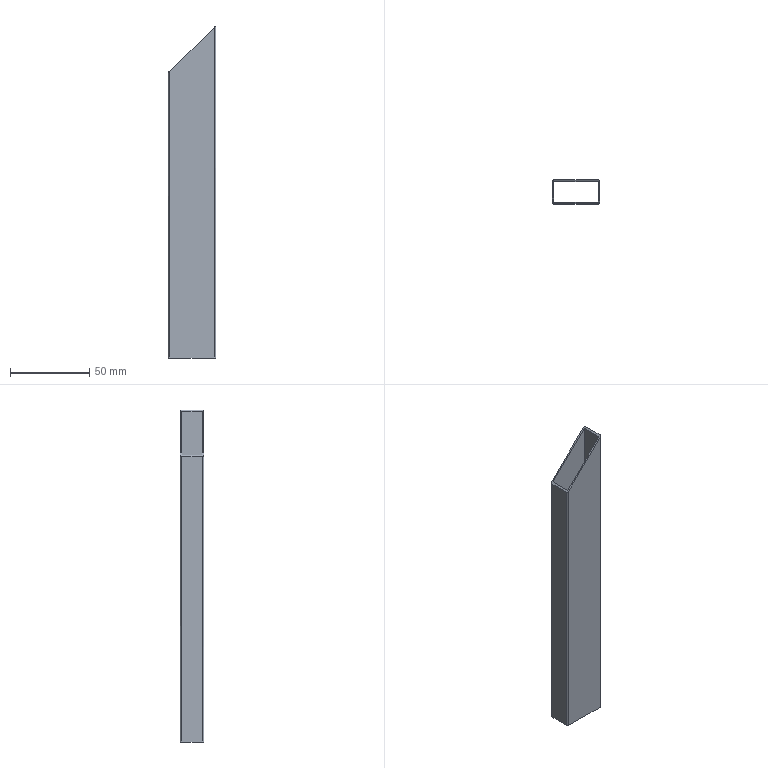Part | STEP file | Q7C1208 | 1 solid | 14 faces | box 30 x 15 x 209.35 mm | volume 16574 mm3 | plane 10 | cylinder 4 | commonest cylinder face diameters 2 x4
STEP:
#1=CARTESIAN_POINT('',(0.,0.,0.));
#2=DIRECTION('',(0.,0.,1.));
#3=DIRECTION('',(1.,0.,0.));
#4=AXIS2_PLACEMENT_3D('',#1,#2,#3);
#5=CARTESIAN_POINT('',(15.,6.5,209.35));
#6=VERTEX_POINT('',#5);
#7=CARTESIAN_POINT('',(14.,7.5,208.371));
#8=VERTEX_POINT('',#7);
#9=CARTESIAN_POINT('',(15.,6.5,209.35));
#10=CARTESIAN_POINT('',(15.,7.086,209.35));
#11=CARTESIAN_POINT('',(14.586,7.5,208.944));
#12=CARTESIAN_POINT('',(14.,7.5,208.371));
#13=(BOUNDED_CURVE()B_SPLINE_CURVE(3,(#9,#10,#11,#12),.UNSPECIFIED.,.F.,.F.)B_SPLINE_CURVE_WITH_KNOTS((4,4),(3.142,4.712),.PIECEWISE_BEZIER_KNOTS.)CURVE()GEOMETRIC_REPRESENTATION_ITEM()RATIONAL_B_SPLINE_CURVE((1.,0.8047,0.8047,1.))REPRESENTATION_ITEM(''));
#14=CARTESIAN_POINT('',(14.,6.5,230.));
#15=DIRECTION('',(0.,0.,-1.));
#16=DIRECTION('',(-1.,0.,0.));
#17=AXIS2_PLACEMENT_3D('',#14,#15,#16);
#18=CYLINDRICAL_SURFACE('',#17,1.);
#19=CARTESIAN_POINT('',(3.142,20.65));
#20=CARTESIAN_POINT('',(3.12,20.65));
#21=CARTESIAN_POINT('',(3.077,20.652));
#22=CARTESIAN_POINT('',(3.01,20.658));
#23=CARTESIAN_POINT('',(2.942,20.669));
#24=CARTESIAN_POINT('',(2.872,20.685));
#25=CARTESIAN_POINT('',(2.801,20.706));
#26=CARTESIAN_POINT('',(2.729,20.732));
#27=CARTESIAN_POINT('',(2.655,20.763));
#28=CARTESIAN_POINT('',(2.581,20.799));
#29=CARTESIAN_POINT('',(2.507,20.84));
#30=CARTESIAN_POINT('',(2.432,20.886));
#31=CARTESIAN_POINT('',(2.356,20.936));
#32=CARTESIAN_POINT('',(2.281,20.991));
#33=CARTESIAN_POINT('',(2.206,21.048));
#34=CARTESIAN_POINT('',(2.131,21.109));
#35=CARTESIAN_POINT('',(2.057,21.171));
#36=CARTESIAN_POINT('',(1.984,21.236));
#37=CARTESIAN_POINT('',(1.912,21.302));
#38=CARTESIAN_POINT('',(1.841,21.368));
#39=CARTESIAN_POINT('',(1.771,21.435));
#40=CARTESIAN_POINT('',(1.702,21.501));
#41=CARTESIAN_POINT('',(1.636,21.566));
#42=CARTESIAN_POINT('',(1.592,21.608));
#43=CARTESIAN_POINT('',(1.571,21.629));
#44=B_SPLINE_CURVE_WITH_KNOTS('',3,(#19,#20,#21,#22,#23,#24,#25,#26,#27,#28,#29,#30,#31,#32,#33,#34,#35,#36,#37,#38,#39,#40,#41,#42,#43),.UNSPECIFIED.,.F.,.F.,(4,1,1,1,1,1,1,1,1,1,1,1,1,1,1,1,1,1,1,1,1,1,4),(3.142,3.213,3.284,3.356,3.427,3.499,3.57,3.641,3.713,3.784,3.856,3.927,3.998,4.07,4.141,4.213,4.284,4.355,4.427,4.498,4.57,4.641,4.712),.QUASI_UNIFORM_KNOTS.);
#45=(GEOMETRIC_REPRESENTATION_CONTEXT(2)PARAMETRIC_REPRESENTATION_CONTEXT()REPRESENTATION_CONTEXT('',''));
#46=DEFINITIONAL_REPRESENTATION('',(#44),#45);
#47=PCURVE('',#18,#46);
#48=CARTESIAN_POINT('',(16.518,298.041,210.835));
#49=DIRECTION('',(-0.6995,0.,0.7146));
#50=DIRECTION('',(0.7146,0.,0.6995));
#51=AXIS2_PLACEMENT_3D('',#48,#49,#50);
#52=PLANE('',#51);
#53=CARTESIAN_POINT('',(-2.124,-291.541));
#54=CARTESIAN_POINT('',(-2.124,-290.955));
#55=CARTESIAN_POINT('',(-2.703,-290.541));
#56=CARTESIAN_POINT('',(-3.523,-290.541));
#57=(BOUNDED_CURVE()B_SPLINE_CURVE(3,(#53,#54,#55,#56),.UNSPECIFIED.,.F.,.F.)B_SPLINE_CURVE_WITH_KNOTS((4,4),(3.142,4.712),.PIECEWISE_BEZIER_KNOTS.)CURVE()GEOMETRIC_REPRESENTATION_ITEM()RATIONAL_B_SPLINE_CURVE((1.,0.8047,0.8047,1.))REPRESENTATION_ITEM(''));
#58=(GEOMETRIC_REPRESENTATION_CONTEXT(2)PARAMETRIC_REPRESENTATION_CONTEXT()REPRESENTATION_CONTEXT('',''));
#59=DEFINITIONAL_REPRESENTATION('',(#57),#58);
#60=PCURVE('',#52,#59);
#61=SURFACE_CURVE('',#13,(#47,#60),.PCURVE_S1.);
#62=EDGE_CURVE('',#6,#8,#61,.T.);
#63=ORIENTED_EDGE('',*,*,#62,.F.);
#64=CARTESIAN_POINT('',(15.,6.5,0.));
#65=VERTEX_POINT('',#64);
#66=CARTESIAN_POINT('',(15.,6.5,230.));
#67=DIRECTION('',(0.,0.,-1.));
#68=VECTOR('',#67,1.);
#69=LINE('',#66,#68);
#70=CARTESIAN_POINT('',(3.142,0.));
#71=DIRECTION('',(0.,1.));
#72=VECTOR('',#71,1.);
#73=LINE('',#70,#72);
#74=(GEOMETRIC_REPRESENTATION_CONTEXT(2)PARAMETRIC_REPRESENTATION_CONTEXT()REPRESENTATION_CONTEXT('',''));
#75=DEFINITIONAL_REPRESENTATION('',(#73),#74);
#76=PCURVE('',#18,#75);
#77=CARTESIAN_POINT('',(15.,6.5,230.));
#78=DIRECTION('',(-1.,0.,0.));
#79=DIRECTION('',(0.,0.,1.));
#80=AXIS2_PLACEMENT_3D('',#77,#78,#79);
#81=PLANE('',#80);
#82=CARTESIAN_POINT('',(0.,0.));
#83=DIRECTION('',(-1.,0.));
#84=VECTOR('',#83,1.);
#85=LINE('',#82,#84);
#86=(GEOMETRIC_REPRESENTATION_CONTEXT(2)PARAMETRIC_REPRESENTATION_CONTEXT()REPRESENTATION_CONTEXT('',''));
#87=DEFINITIONAL_REPRESENTATION('',(#85),#86);
#88=PCURVE('',#81,#87);
#89=SURFACE_CURVE('',#69,(#76,#88),.PCURVE_S1.);
#90=EDGE_CURVE('',#6,#65,#89,.T.);
#91=ORIENTED_EDGE('',*,*,#90,.T.);
#92=CARTESIAN_POINT('',(14.,7.5,0.));
#93=VERTEX_POINT('',#92);
#94=CARTESIAN_POINT('',(14.,6.5,0.));
#95=DIRECTION('',(0.,0.,1.));
#96=DIRECTION('',(-1.,0.,0.));
#97=AXIS2_PLACEMENT_3D('',#94,#95,#96);
#98=CIRCLE('',#97,1.);
#99=CARTESIAN_POINT('',(6.283,230.));
#100=DIRECTION('',(-1.,0.));
#101=VECTOR('',#100,1.);
#102=LINE('',#99,#101);
#103=(GEOMETRIC_REPRESENTATION_CONTEXT(2)PARAMETRIC_REPRESENTATION_CONTEXT()REPRESENTATION_CONTEXT('',''));
#104=DEFINITIONAL_REPRESENTATION('',(#102),#103);
#105=PCURVE('',#18,#104);
#106=CARTESIAN_POINT('',(14.,6.5,0.));
#107=DIRECTION('',(0.,0.,-1.));
#108=DIRECTION('',(-1.,0.,0.));
#109=AXIS2_PLACEMENT_3D('',#106,#107,#108);
#110=PLANE('',#109);
#111=CARTESIAN_POINT('',(1.,0.));
#112=CARTESIAN_POINT('',(1.,-1.732));
#113=CARTESIAN_POINT('',(-0.5,-0.866));
#114=CARTESIAN_POINT('',(-2.,0.));
#115=CARTESIAN_POINT('',(-0.5,0.866));
#116=CARTESIAN_POINT('',(1.,1.732));
#117=CARTESIAN_POINT('',(1.,0.));
#118=(BOUNDED_CURVE()B_SPLINE_CURVE(2,(#111,#112,#113,#114,#115,#116,#117),.UNSPECIFIED.,.T.,.F.)B_SPLINE_CURVE_WITH_KNOTS((1,2,2,2,2,1),(-2.094,0.,2.094,4.189,6.283,8.378),.UNSPECIFIED.)CURVE()GEOMETRIC_REPRESENTATION_ITEM()RATIONAL_B_SPLINE_CURVE((1.,0.5,1.,0.5,1.,0.5,1.))REPRESENTATION_ITEM(''));
#119=(GEOMETRIC_REPRESENTATION_CONTEXT(2)PARAMETRIC_REPRESENTATION_CONTEXT()REPRESENTATION_CONTEXT('',''));
#120=DEFINITIONAL_REPRESENTATION('',(#118),#119);
#121=PCURVE('',#110,#120);
#122=SURFACE_CURVE('',#98,(#105,#121),.PCURVE_S1.);
#123=EDGE_CURVE('',#65,#93,#122,.T.);
#124=ORIENTED_EDGE('',*,*,#123,.T.);
#125=CARTESIAN_POINT('',(14.,7.5,230.));
#126=DIRECTION('',(0.,0.,-1.));
#127=VECTOR('',#126,1.);
#128=LINE('',#125,#127);
#129=CARTESIAN_POINT('',(1.571,0.));
#130=DIRECTION('',(0.,1.));
#131=VECTOR('',#130,1.);
#132=LINE('',#129,#131);
#133=(GEOMETRIC_REPRESENTATION_CONTEXT(2)PARAMETRIC_REPRESENTATION_CONTEXT()REPRESENTATION_CONTEXT('',''));
#134=DEFINITIONAL_REPRESENTATION('',(#132),#133);
#135=PCURVE('',#18,#134);
#136=CARTESIAN_POINT('',(-14.,7.5,230.));
#137=DIRECTION('',(0.,-1.,0.));
#138=DIRECTION('',(0.,0.,-1.));
#139=AXIS2_PLACEMENT_3D('',#136,#137,#138);
#140=PLANE('',#139);
#141=CARTESIAN_POINT('',(0.,28.));
#142=DIRECTION('',(1.,0.));
#143=VECTOR('',#142,1.);
#144=LINE('',#141,#143);
#145=(GEOMETRIC_REPRESENTATION_CONTEXT(2)PARAMETRIC_REPRESENTATION_CONTEXT()REPRESENTATION_CONTEXT('',''));
#146=DEFINITIONAL_REPRESENTATION('',(#144),#145);
#147=PCURVE('',#140,#146);
#148=SURFACE_CURVE('',#128,(#135,#147),.PCURVE_S1.);
#149=EDGE_CURVE('',#8,#93,#148,.T.);
#150=ORIENTED_EDGE('',*,*,#149,.F.);
#151=EDGE_LOOP('',(#63,#91,#124,#150));
#152=FACE_BOUND('',#151,.T.);
#153=ADVANCED_FACE('',(#152),#18,.T.);
#154=CARTESIAN_POINT('',(-14.,7.5,180.963));
#155=VERTEX_POINT('',#154);
#156=CARTESIAN_POINT('',(10.513,7.5,204.958));
#157=DIRECTION('',(-0.7146,0.,-0.6995));
#158=VECTOR('',#157,1.);
#159=LINE('',#156,#158);
#160=CARTESIAN_POINT('',(25.042,24.513));
#161=DIRECTION('',(0.6995,-0.7146));
#162=VECTOR('',#161,1.);
#163=LINE('',#160,#162);
#164=(GEOMETRIC_REPRESENTATION_CONTEXT(2)PARAMETRIC_REPRESENTATION_CONTEXT()REPRESENTATION_CONTEXT('',''));
#165=DEFINITIONAL_REPRESENTATION('',(#163),#164);
#166=PCURVE('',#140,#165);
#167=CARTESIAN_POINT('',(-8.403,-290.541));
#168=DIRECTION('',(-1.,0.));
#169=VECTOR('',#168,1.);
#170=LINE('',#167,#169);
#171=(GEOMETRIC_REPRESENTATION_CONTEXT(2)PARAMETRIC_REPRESENTATION_CONTEXT()REPRESENTATION_CONTEXT('',''));
#172=DEFINITIONAL_REPRESENTATION('',(#170),#171);
#173=PCURVE('',#52,#172);
#174=SURFACE_CURVE('',#159,(#166,#173),.PCURVE_S1.);
#175=EDGE_CURVE('',#8,#155,#174,.T.);
#176=ORIENTED_EDGE('',*,*,#175,.F.);
#177=ORIENTED_EDGE('',*,*,#149,.T.);
#178=CARTESIAN_POINT('',(-14.,7.5,0.));
#179=VERTEX_POINT('',#178);
#180=CARTESIAN_POINT('',(-14.,7.5,0.));
#181=DIRECTION('',(-1.,0.,0.));
#182=VECTOR('',#181,1.);
#183=LINE('',#180,#182);
#184=CARTESIAN_POINT('',(230.,0.));
#185=DIRECTION('',(0.,-1.));
#186=VECTOR('',#185,1.);
#187=LINE('',#184,#186);
#188=(GEOMETRIC_REPRESENTATION_CONTEXT(2)PARAMETRIC_REPRESENTATION_CONTEXT()REPRESENTATION_CONTEXT('',''));
#189=DEFINITIONAL_REPRESENTATION('',(#187),#188);
#190=PCURVE('',#140,#189);
#191=CARTESIAN_POINT('',(28.,1.));
#192=DIRECTION('',(1.,0.));
#193=VECTOR('',#192,1.);
#194=LINE('',#191,#193);
#195=(GEOMETRIC_REPRESENTATION_CONTEXT(2)PARAMETRIC_REPRESENTATION_CONTEXT()REPRESENTATION_CONTEXT('',''));
#196=DEFINITIONAL_REPRESENTATION('',(#194),#195);
#197=PCURVE('',#110,#196);
#198=SURFACE_CURVE('',#183,(#190,#197),.PCURVE_S1.);
#199=EDGE_CURVE('',#93,#179,#198,.T.);
#200=ORIENTED_EDGE('',*,*,#199,.T.);
#201=CARTESIAN_POINT('',(-14.,7.5,230.));
#202=DIRECTION('',(0.,0.,-1.));
#203=VECTOR('',#202,1.);
#204=LINE('',#201,#203);
#205=CARTESIAN_POINT('',(0.,0.));
#206=DIRECTION('',(1.,0.));
#207=VECTOR('',#206,1.);
#208=LINE('',#205,#207);
#209=(GEOMETRIC_REPRESENTATION_CONTEXT(2)PARAMETRIC_REPRESENTATION_CONTEXT()REPRESENTATION_CONTEXT('',''));
#210=DEFINITIONAL_REPRESENTATION('',(#208),#209);
#211=PCURVE('',#140,#210);
#212=CARTESIAN_POINT('',(-14.,6.5,230.));
#213=DIRECTION('',(0.,0.,-1.));
#214=DIRECTION('',(-1.,0.,0.));
#215=AXIS2_PLACEMENT_3D('',#212,#213,#214);
#216=CYLINDRICAL_SURFACE('',#215,1.);
#217=CARTESIAN_POINT('',(1.571,0.));
#218=DIRECTION('',(0.,1.));
#219=VECTOR('',#218,1.);
#220=LINE('',#217,#219);
#221=(GEOMETRIC_REPRESENTATION_CONTEXT(2)PARAMETRIC_REPRESENTATION_CONTEXT()REPRESENTATION_CONTEXT('',''));
#222=DEFINITIONAL_REPRESENTATION('',(#220),#221);
#223=PCURVE('',#216,#222);
#224=SURFACE_CURVE('',#204,(#211,#223),.PCURVE_S1.);
#225=EDGE_CURVE('',#155,#179,#224,.T.);
#226=ORIENTED_EDGE('',*,*,#225,.F.);
#227=EDGE_LOOP('',(#176,#177,#200,#226));
#228=FACE_BOUND('',#227,.T.);
#229=ADVANCED_FACE('',(#228),#140,.F.);
#230=CARTESIAN_POINT('',(-15.,6.5,179.984));
#231=VERTEX_POINT('',#230);
#232=CARTESIAN_POINT('',(-14.,7.5,180.963));
#233=CARTESIAN_POINT('',(-14.586,7.5,180.389));
#234=CARTESIAN_POINT('',(-15.,7.086,179.984));
#235=CARTESIAN_POINT('',(-15.,6.5,179.984));
#236=(BOUNDED_CURVE()B_SPLINE_CURVE(3,(#232,#233,#234,#235),.UNSPECIFIED.,.F.,.F.)B_SPLINE_CURVE_WITH_KNOTS((4,4),(4.712,6.283),.PIECEWISE_BEZIER_KNOTS.)CURVE()GEOMETRIC_REPRESENTATION_ITEM()RATIONAL_B_SPLINE_CURVE((1.,0.8047,0.8047,1.))REPRESENTATION_ITEM(''));
#237=CARTESIAN_POINT('',(1.571,49.037));
#238=CARTESIAN_POINT('',(1.549,49.058));
#239=CARTESIAN_POINT('',(1.506,49.101));
#240=CARTESIAN_POINT('',(1.439,49.166));
#241=CARTESIAN_POINT('',(1.371,49.232));
#242=CARTESIAN_POINT('',(1.301,49.298));
#243=CARTESIAN_POINT('',(1.23,49.365));
#244=CARTESIAN_POINT('',(1.158,49.431));
#245=CARTESIAN_POINT('',(1.085,49.495));
#246=CARTESIAN_POINT('',(1.01,49.558));
#247=CARTESIAN_POINT('',(0.9358,49.619));
#248=CARTESIAN_POINT('',(0.8607,49.676));
#249=CARTESIAN_POINT('',(0.7854,49.73));
#250=CARTESIAN_POINT('',(0.7101,49.78));
#251=CARTESIAN_POINT('',(0.635,49.826));
#252=CARTESIAN_POINT('',(0.5603,49.867));
#253=CARTESIAN_POINT('',(0.4863,49.904));
#254=CARTESIAN_POINT('',(0.413,49.935));
#255=CARTESIAN_POINT('',(0.3408,49.961));
#256=CARTESIAN_POINT('',(0.2697,49.982));
#257=CARTESIAN_POINT('',(0.2,49.997));
#258=CARTESIAN_POINT('',(0.1316,50.008));
#259=CARTESIAN_POINT('',(0.06485,50.015));
#260=CARTESIAN_POINT('',(0.02143,50.016));
#261=CARTESIAN_POINT('',(0.,50.016));
#262=B_SPLINE_CURVE_WITH_KNOTS('',3,(#237,#238,#239,#240,#241,#242,#243,#244,#245,#246,#247,#248,#249,#250,#251,#252,#253,#254,#255,#256,#257,#258,#259,#260,#261),.UNSPECIFIED.,.F.,.F.,(4,1,1,1,1,1,1,1,1,1,1,1,1,1,1,1,1,1,1,1,1,1,4),(4.712,4.784,4.855,4.927,4.998,5.069,5.141,5.212,5.284,5.355,5.426,5.498,5.569,5.641,5.712,5.783,5.855,5.926,5.998,6.069,6.14,6.212,6.283),.QUASI_UNIFORM_KNOTS.);
#263=(GEOMETRIC_REPRESENTATION_CONTEXT(2)PARAMETRIC_REPRESENTATION_CONTEXT()REPRESENTATION_CONTEXT('',''));
#264=DEFINITIONAL_REPRESENTATION('',(#262),#263);
#265=PCURVE('',#216,#264);
#266=CARTESIAN_POINT('',(-42.705,-290.541));
#267=CARTESIAN_POINT('',(-43.525,-290.541));
#268=CARTESIAN_POINT('',(-44.104,-290.955));
#269=CARTESIAN_POINT('',(-44.104,-291.541));
#270=(BOUNDED_CURVE()B_SPLINE_CURVE(3,(#266,#267,#268,#269),.UNSPECIFIED.,.F.,.F.)B_SPLINE_CURVE_WITH_KNOTS((4,4),(4.712,6.283),.PIECEWISE_BEZIER_KNOTS.)CURVE()GEOMETRIC_REPRESENTATION_ITEM()RATIONAL_B_SPLINE_CURVE((1.,0.8047,0.8047,1.))REPRESENTATION_ITEM(''));
#271=(GEOMETRIC_REPRESENTATION_CONTEXT(2)PARAMETRIC_REPRESENTATION_CONTEXT()REPRESENTATION_CONTEXT('',''));
#272=DEFINITIONAL_REPRESENTATION('',(#270),#271);
#273=PCURVE('',#52,#272);
#274=SURFACE_CURVE('',#236,(#265,#273),.PCURVE_S1.);
#275=EDGE_CURVE('',#155,#231,#274,.T.);
#276=ORIENTED_EDGE('',*,*,#275,.F.);
#277=ORIENTED_EDGE('',*,*,#225,.T.);
#278=CARTESIAN_POINT('',(-15.,6.5,0.));
#279=VERTEX_POINT('',#278);
#280=CARTESIAN_POINT('',(-14.,6.5,0.));
#281=DIRECTION('',(0.,0.,1.));
#282=DIRECTION('',(1.,0.,0.));
#283=AXIS2_PLACEMENT_3D('',#280,#281,#282);
#284=CIRCLE('',#283,1.);
#285=CARTESIAN_POINT('',(3.142,230.));
#286=DIRECTION('',(-1.,0.));
#287=VECTOR('',#286,1.);
#288=LINE('',#285,#287);
#289=(GEOMETRIC_REPRESENTATION_CONTEXT(2)PARAMETRIC_REPRESENTATION_CONTEXT()REPRESENTATION_CONTEXT('',''));
#290=DEFINITIONAL_REPRESENTATION('',(#288),#289);
#291=PCURVE('',#216,#290);
#292=CARTESIAN_POINT('',(27.,0.));
#293=CARTESIAN_POINT('',(27.,1.732));
#294=CARTESIAN_POINT('',(28.5,0.866));
#295=CARTESIAN_POINT('',(30.,0.));
#296=CARTESIAN_POINT('',(28.5,-0.866));
#297=CARTESIAN_POINT('',(27.,-1.732));
#298=CARTESIAN_POINT('',(27.,0.));
#299=(BOUNDED_CURVE()B_SPLINE_CURVE(2,(#292,#293,#294,#295,#296,#297,#298),.UNSPECIFIED.,.T.,.F.)B_SPLINE_CURVE_WITH_KNOTS((1,2,2,2,2,1),(-2.094,0.,2.094,4.189,6.283,8.378),.UNSPECIFIED.)CURVE()GEOMETRIC_REPRESENTATION_ITEM()RATIONAL_B_SPLINE_CURVE((1.,0.5,1.,0.5,1.,0.5,1.))REPRESENTATION_ITEM(''));
#300=(GEOMETRIC_REPRESENTATION_CONTEXT(2)PARAMETRIC_REPRESENTATION_CONTEXT()REPRESENTATION_CONTEXT('',''));
#301=DEFINITIONAL_REPRESENTATION('',(#299),#300);
#302=PCURVE('',#110,#301);
#303=SURFACE_CURVE('',#284,(#291,#302),.PCURVE_S1.);
#304=EDGE_CURVE('',#179,#279,#303,.T.);
#305=ORIENTED_EDGE('',*,*,#304,.T.);
#306=CARTESIAN_POINT('',(-15.,6.5,230.));
#307=DIRECTION('',(0.,0.,-1.));
#308=VECTOR('',#307,1.);
#309=LINE('',#306,#308);
#310=CARTESIAN_POINT('',(0.,0.));
#311=DIRECTION('',(0.,1.));
#312=VECTOR('',#311,1.);
#313=LINE('',#310,#312);
#314=(GEOMETRIC_REPRESENTATION_CONTEXT(2)PARAMETRIC_REPRESENTATION_CONTEXT()REPRESENTATION_CONTEXT('',''));
#315=DEFINITIONAL_REPRESENTATION('',(#313),#314);
#316=PCURVE('',#216,#315);
#317=CARTESIAN_POINT('',(-15.,6.5,230.));
#318=DIRECTION('',(1.,0.,0.));
#319=DIRECTION('',(0.,1.,0.));
#320=AXIS2_PLACEMENT_3D('',#317,#318,#319);
#321=PLANE('',#320);
#322=CARTESIAN_POINT('',(0.,0.));
#323=DIRECTION('',(0.,-1.));
#324=VECTOR('',#323,1.);
#325=LINE('',#322,#324);
#326=(GEOMETRIC_REPRESENTATION_CONTEXT(2)PARAMETRIC_REPRESENTATION_CONTEXT()REPRESENTATION_CONTEXT('',''));
#327=DEFINITIONAL_REPRESENTATION('',(#325),#326);
#328=PCURVE('',#321,#327);
#329=SURFACE_CURVE('',#309,(#316,#328),.PCURVE_S1.);
#330=EDGE_CURVE('',#231,#279,#329,.T.);
#331=ORIENTED_EDGE('',*,*,#330,.F.);
#332=EDGE_LOOP('',(#276,#277,#305,#331));
#333=FACE_BOUND('',#332,.T.);
#334=ADVANCED_FACE('',(#333),#216,.T.);
#335=CARTESIAN_POINT('',(-15.,-6.5,179.984));
#336=VERTEX_POINT('',#335);
#337=CARTESIAN_POINT('',(-15.,6.5,179.984));
#338=DIRECTION('',(0.,-1.,0.));
#339=VECTOR('',#338,1.);
#340=LINE('',#337,#339);
#341=CARTESIAN_POINT('',(0.,-50.016));
#342=DIRECTION('',(-1.,0.));
#343=VECTOR('',#342,1.);
#344=LINE('',#341,#343);
#345=(GEOMETRIC_REPRESENTATION_CONTEXT(2)PARAMETRIC_REPRESENTATION_CONTEXT()REPRESENTATION_CONTEXT('',''));
#346=DEFINITIONAL_REPRESENTATION('',(#344),#345);
#347=PCURVE('',#321,#346);
#348=CARTESIAN_POINT('',(-44.104,-291.541));
#349=DIRECTION('',(0.,-1.));
#350=VECTOR('',#349,1.);
#351=LINE('',#348,#350);
#352=(GEOMETRIC_REPRESENTATION_CONTEXT(2)PARAMETRIC_REPRESENTATION_CONTEXT()REPRESENTATION_CONTEXT('',''));
#353=DEFINITIONAL_REPRESENTATION('',(#351),#352);
#354=PCURVE('',#52,#353);
#355=SURFACE_CURVE('',#340,(#347,#354),.PCURVE_S1.);
#356=EDGE_CURVE('',#231,#336,#355,.T.);
#357=ORIENTED_EDGE('',*,*,#356,.F.);
#358=ORIENTED_EDGE('',*,*,#330,.T.);
#359=CARTESIAN_POINT('',(-15.,-6.5,0.));
#360=VERTEX_POINT('',#359);
#361=CARTESIAN_POINT('',(-15.,6.5,0.));
#362=DIRECTION('',(0.,-1.,0.));
#363=VECTOR('',#362,1.);
#364=LINE('',#361,#363);
#365=CARTESIAN_POINT('',(0.,-230.));
#366=DIRECTION('',(-1.,0.));
#367=VECTOR('',#366,1.);
#368=LINE('',#365,#367);
#369=(GEOMETRIC_REPRESENTATION_CONTEXT(2)PARAMETRIC_REPRESENTATION_CONTEXT()REPRESENTATION_CONTEXT('',''));
#370=DEFINITIONAL_REPRESENTATION('',(#368),#369);
#371=PCURVE('',#321,#370);
#372=CARTESIAN_POINT('',(29.,0.));
#373=DIRECTION('',(0.,-1.));
#374=VECTOR('',#373,1.);
#375=LINE('',#372,#374);
#376=(GEOMETRIC_REPRESENTATION_CONTEXT(2)PARAMETRIC_REPRESENTATION_CONTEXT()REPRESENTATION_CONTEXT('',''));
#377=DEFINITIONAL_REPRESENTATION('',(#375),#376);
#378=PCURVE('',#110,#377);
#379=SURFACE_CURVE('',#364,(#371,#378),.PCURVE_S1.);
#380=EDGE_CURVE('',#279,#360,#379,.T.);
#381=ORIENTED_EDGE('',*,*,#380,.T.);
#382=CARTESIAN_POINT('',(-15.,-6.5,230.));
#383=DIRECTION('',(0.,0.,-1.));
#384=VECTOR('',#383,1.);
#385=LINE('',#382,#384);
#386=CARTESIAN_POINT('',(-13.,0.));
#387=DIRECTION('',(0.,-1.));
#388=VECTOR('',#387,1.);
#389=LINE('',#386,#388);
#390=(GEOMETRIC_REPRESENTATION_CONTEXT(2)PARAMETRIC_REPRESENTATION_CONTEXT()REPRESENTATION_CONTEXT('',''));
#391=DEFINITIONAL_REPRESENTATION('',(#389),#390);
#392=PCURVE('',#321,#391);
#393=CARTESIAN_POINT('',(-14.,-6.5,230.));
#394=DIRECTION('',(0.,0.,-1.));
#395=DIRECTION('',(-1.,0.,0.));
#396=AXIS2_PLACEMENT_3D('',#393,#394,#395);
#397=CYLINDRICAL_SURFACE('',#396,1.);
#398=CARTESIAN_POINT('',(6.283,0.));
#399=DIRECTION('',(0.,1.));
#400=VECTOR('',#399,1.);
#401=LINE('',#398,#400);
#402=(GEOMETRIC_REPRESENTATION_CONTEXT(2)PARAMETRIC_REPRESENTATION_CONTEXT()REPRESENTATION_CONTEXT('',''));
#403=DEFINITIONAL_REPRESENTATION('',(#401),#402);
#404=PCURVE('',#397,#403);
#405=SURFACE_CURVE('',#385,(#392,#404),.PCURVE_S1.);
#406=EDGE_CURVE('',#336,#360,#405,.T.);
#407=ORIENTED_EDGE('',*,*,#406,.F.);
#408=EDGE_LOOP('',(#357,#358,#381,#407));
#409=FACE_BOUND('',#408,.T.);
#410=ADVANCED_FACE('',(#409),#321,.F.);
#411=CARTESIAN_POINT('',(-14.,-7.5,180.963));
#412=VERTEX_POINT('',#411);
#413=CARTESIAN_POINT('',(-15.,-6.5,179.984));
#414=CARTESIAN_POINT('',(-15.,-7.086,179.984));
#415=CARTESIAN_POINT('',(-14.586,-7.5,180.389));
#416=CARTESIAN_POINT('',(-14.,-7.5,180.963));
#417=(BOUNDED_CURVE()B_SPLINE_CURVE(3,(#413,#414,#415,#416),.UNSPECIFIED.,.F.,.F.)B_SPLINE_CURVE_WITH_KNOTS((4,4),(0.,1.571),.PIECEWISE_BEZIER_KNOTS.)CURVE()GEOMETRIC_REPRESENTATION_ITEM()RATIONAL_B_SPLINE_CURVE((1.,0.8047,0.8047,1.))REPRESENTATION_ITEM(''));
#418=CARTESIAN_POINT('',(6.283,50.016));
#419=CARTESIAN_POINT('',(6.262,50.016));
#420=CARTESIAN_POINT('',(6.218,50.015));
#421=CARTESIAN_POINT('',(6.152,50.008));
#422=CARTESIAN_POINT('',(6.083,49.997));
#423=CARTESIAN_POINT('',(6.013,49.982));
#424=CARTESIAN_POINT('',(5.942,49.961));
#425=CARTESIAN_POINT('',(5.87,49.935));
#426=CARTESIAN_POINT('',(5.797,49.904));
#427=CARTESIAN_POINT('',(5.723,49.867));
#428=CARTESIAN_POINT('',(5.648,49.826));
#429=CARTESIAN_POINT('',(5.573,49.78));
#430=CARTESIAN_POINT('',(5.498,49.73));
#431=CARTESIAN_POINT('',(5.422,49.676));
#432=CARTESIAN_POINT('',(5.347,49.619));
#433=CARTESIAN_POINT('',(5.273,49.558));
#434=CARTESIAN_POINT('',(5.199,49.495));
#435=CARTESIAN_POINT('',(5.125,49.431));
#436=CARTESIAN_POINT('',(5.053,49.365));
#437=CARTESIAN_POINT('',(4.982,49.298));
#438=CARTESIAN_POINT('',(4.912,49.232));
#439=CARTESIAN_POINT('',(4.844,49.166));
#440=CARTESIAN_POINT('',(4.777,49.101));
#441=CARTESIAN_POINT('',(4.734,49.058));
#442=CARTESIAN_POINT('',(4.712,49.037));
#443=B_SPLINE_CURVE_WITH_KNOTS('',3,(#418,#419,#420,#421,#422,#423,#424,#425,#426,#427,#428,#429,#430,#431,#432,#433,#434,#435,#436,#437,#438,#439,#440,#441,#442),.UNSPECIFIED.,.F.,.F.,(4,1,1,1,1,1,1,1,1,1,1,1,1,1,1,1,1,1,1,1,1,1,4),(0.,0.0714,0.1428,0.2142,0.2856,0.357,0.4284,0.4998,0.5712,0.6426,0.714,0.7854,0.8568,0.9282,0.9996,1.071,1.142,1.214,1.285,1.357,1.428,1.499,1.571),.QUASI_UNIFORM_KNOTS.);
#444=(GEOMETRIC_REPRESENTATION_CONTEXT(2)PARAMETRIC_REPRESENTATION_CONTEXT()REPRESENTATION_CONTEXT('',''));
#445=DEFINITIONAL_REPRESENTATION('',(#443),#444);
#446=PCURVE('',#397,#445);
#447=CARTESIAN_POINT('',(-44.104,-304.541));
#448=CARTESIAN_POINT('',(-44.104,-305.127));
#449=CARTESIAN_POINT('',(-43.525,-305.541));
#450=CARTESIAN_POINT('',(-42.705,-305.541));
#451=(BOUNDED_CURVE()B_SPLINE_CURVE(3,(#447,#448,#449,#450),.UNSPECIFIED.,.F.,.F.)B_SPLINE_CURVE_WITH_KNOTS((4,4),(0.,1.571),.PIECEWISE_BEZIER_KNOTS.)CURVE()GEOMETRIC_REPRESENTATION_ITEM()RATIONAL_B_SPLINE_CURVE((1.,0.8047,0.8047,1.))REPRESENTATION_ITEM(''));
#452=(GEOMETRIC_REPRESENTATION_CONTEXT(2)PARAMETRIC_REPRESENTATION_CONTEXT()REPRESENTATION_CONTEXT('',''));
#453=DEFINITIONAL_REPRESENTATION('',(#451),#452);
#454=PCURVE('',#52,#453);
#455=SURFACE_CURVE('',#417,(#446,#454),.PCURVE_S1.);
#456=EDGE_CURVE('',#336,#412,#455,.T.);
#457=ORIENTED_EDGE('',*,*,#456,.F.);
#458=ORIENTED_EDGE('',*,*,#406,.T.);
#459=CARTESIAN_POINT('',(-14.,-7.5,0.));
#460=VERTEX_POINT('',#459);
#461=CARTESIAN_POINT('',(-14.,-6.5,0.));
#462=DIRECTION('',(0.,0.,1.));
#463=DIRECTION('',(1.,0.,0.));
#464=AXIS2_PLACEMENT_3D('',#461,#462,#463);
#465=CIRCLE('',#464,1.);
#466=CARTESIAN_POINT('',(9.425,230.));
#467=DIRECTION('',(-1.,0.));
#468=VECTOR('',#467,1.);
#469=LINE('',#466,#468);
#470=(GEOMETRIC_REPRESENTATION_CONTEXT(2)PARAMETRIC_REPRESENTATION_CONTEXT()REPRESENTATION_CONTEXT('',''));
#471=DEFINITIONAL_REPRESENTATION('',(#469),#470);
#472=PCURVE('',#397,#471);
#473=CARTESIAN_POINT('',(27.,-13.));
#474=CARTESIAN_POINT('',(27.,-11.268));
#475=CARTESIAN_POINT('',(28.5,-12.134));
#476=CARTESIAN_POINT('',(30.,-13.));
#477=CARTESIAN_POINT('',(28.5,-13.866));
#478=CARTESIAN_POINT('',(27.,-14.732));
#479=CARTESIAN_POINT('',(27.,-13.));
#480=(BOUNDED_CURVE()B_SPLINE_CURVE(2,(#473,#474,#475,#476,#477,#478,#479),.UNSPECIFIED.,.T.,.F.)B_SPLINE_CURVE_WITH_KNOTS((1,2,2,2,2,1),(-2.094,0.,2.094,4.189,6.283,8.378),.UNSPECIFIED.)CURVE()GEOMETRIC_REPRESENTATION_ITEM()RATIONAL_B_SPLINE_CURVE((1.,0.5,1.,0.5,1.,0.5,1.))REPRESENTATION_ITEM(''));
#481=(GEOMETRIC_REPRESENTATION_CONTEXT(2)PARAMETRIC_REPRESENTATION_CONTEXT()REPRESENTATION_CONTEXT('',''));
#482=DEFINITIONAL_REPRESENTATION('',(#480),#481);
#483=PCURVE('',#110,#482);
#484=SURFACE_CURVE('',#465,(#472,#483),.PCURVE_S1.);
#485=EDGE_CURVE('',#360,#460,#484,.T.);
#486=ORIENTED_EDGE('',*,*,#485,.T.);
#487=CARTESIAN_POINT('',(-14.,-7.5,230.));
#488=DIRECTION('',(0.,0.,-1.));
#489=VECTOR('',#488,1.);
#490=LINE('',#487,#489);
#491=CARTESIAN_POINT('',(4.712,0.));
#492=DIRECTION('',(0.,1.));
#493=VECTOR('',#492,1.);
#494=LINE('',#491,#493);
#495=(GEOMETRIC_REPRESENTATION_CONTEXT(2)PARAMETRIC_REPRESENTATION_CONTEXT()REPRESENTATION_CONTEXT('',''));
#496=DEFINITIONAL_REPRESENTATION('',(#494),#495);
#497=PCURVE('',#397,#496);
#498=CARTESIAN_POINT('',(-14.,-7.5,230.));
#499=DIRECTION('',(0.,1.,0.));
#500=DIRECTION('',(0.,0.,1.));
#501=AXIS2_PLACEMENT_3D('',#498,#499,#500);
#502=PLANE('',#501);
#503=CARTESIAN_POINT('',(0.,0.));
#504=DIRECTION('',(-1.,0.));
#505=VECTOR('',#504,1.);
#506=LINE('',#503,#505);
#507=(GEOMETRIC_REPRESENTATION_CONTEXT(2)PARAMETRIC_REPRESENTATION_CONTEXT()REPRESENTATION_CONTEXT('',''));
#508=DEFINITIONAL_REPRESENTATION('',(#506),#507);
#509=PCURVE('',#502,#508);
#510=SURFACE_CURVE('',#490,(#497,#509),.PCURVE_S1.);
#511=EDGE_CURVE('',#412,#460,#510,.T.);
#512=ORIENTED_EDGE('',*,*,#511,.F.);
#513=EDGE_LOOP('',(#457,#458,#486,#512));
#514=FACE_BOUND('',#513,.T.);
#515=ADVANCED_FACE('',(#514),#397,.T.);
#516=CARTESIAN_POINT('',(14.,-7.5,208.371));
#517=VERTEX_POINT('',#516);
#518=CARTESIAN_POINT('',(10.513,-7.5,204.958));
#519=DIRECTION('',(0.7146,0.,0.6995));
#520=VECTOR('',#519,1.);
#521=LINE('',#518,#520);
#522=CARTESIAN_POINT('',(-25.042,24.513));
#523=DIRECTION('',(0.6995,0.7146));
#524=VECTOR('',#523,1.);
#525=LINE('',#522,#524);
#526=(GEOMETRIC_REPRESENTATION_CONTEXT(2)PARAMETRIC_REPRESENTATION_CONTEXT()REPRESENTATION_CONTEXT('',''));
#527=DEFINITIONAL_REPRESENTATION('',(#525),#526);
#528=PCURVE('',#502,#527);
#529=CARTESIAN_POINT('',(-8.403,-305.541));
#530=DIRECTION('',(1.,0.));
#531=VECTOR('',#530,1.);
#532=LINE('',#529,#531);
#533=(GEOMETRIC_REPRESENTATION_CONTEXT(2)PARAMETRIC_REPRESENTATION_CONTEXT()REPRESENTATION_CONTEXT('',''));
#534=DEFINITIONAL_REPRESENTATION('',(#532),#533);
#535=PCURVE('',#52,#534);
#536=SURFACE_CURVE('',#521,(#528,#535),.PCURVE_S1.);
#537=EDGE_CURVE('',#412,#517,#536,.T.);
#538=ORIENTED_EDGE('',*,*,#537,.F.);
#539=ORIENTED_EDGE('',*,*,#511,.T.);
#540=CARTESIAN_POINT('',(14.,-7.5,0.));
#541=VERTEX_POINT('',#540);
#542=CARTESIAN_POINT('',(-14.,-7.5,0.));
#543=DIRECTION('',(1.,0.,0.));
#544=VECTOR('',#543,1.);
#545=LINE('',#542,#544);
#546=CARTESIAN_POINT('',(-230.,0.));
#547=DIRECTION('',(0.,1.));
#548=VECTOR('',#547,1.);
#549=LINE('',#546,#548);
#550=(GEOMETRIC_REPRESENTATION_CONTEXT(2)PARAMETRIC_REPRESENTATION_CONTEXT()REPRESENTATION_CONTEXT('',''));
#551=DEFINITIONAL_REPRESENTATION('',(#549),#550);
#552=PCURVE('',#502,#551);
#553=CARTESIAN_POINT('',(28.,-14.));
#554=DIRECTION('',(-1.,0.));
#555=VECTOR('',#554,1.);
#556=LINE('',#553,#555);
#557=(GEOMETRIC_REPRESENTATION_CONTEXT(2)PARAMETRIC_REPRESENTATION_CONTEXT()REPRESENTATION_CONTEXT('',''));
#558=DEFINITIONAL_REPRESENTATION('',(#556),#557);
#559=PCURVE('',#110,#558);
#560=SURFACE_CURVE('',#545,(#552,#559),.PCURVE_S1.);
#561=EDGE_CURVE('',#460,#541,#560,.T.);
#562=ORIENTED_EDGE('',*,*,#561,.T.);
#563=CARTESIAN_POINT('',(14.,-7.5,230.));
#564=DIRECTION('',(0.,0.,-1.));
#565=VECTOR('',#564,1.);
#566=LINE('',#563,#565);
#567=CARTESIAN_POINT('',(0.,28.));
#568=DIRECTION('',(-1.,0.));
#569=VECTOR('',#568,1.);
#570=LINE('',#567,#569);
#571=(GEOMETRIC_REPRESENTATION_CONTEXT(2)PARAMETRIC_REPRESENTATION_CONTEXT()REPRESENTATION_CONTEXT('',''));
#572=DEFINITIONAL_REPRESENTATION('',(#570),#571);
#573=PCURVE('',#502,#572);
#574=CARTESIAN_POINT('',(14.,-6.5,230.));
#575=DIRECTION('',(0.,0.,-1.));
#576=DIRECTION('',(-1.,0.,0.));
#577=AXIS2_PLACEMENT_3D('',#574,#575,#576);
#578=CYLINDRICAL_SURFACE('',#577,1.);
#579=CARTESIAN_POINT('',(4.712,0.));
#580=DIRECTION('',(0.,1.));
#581=VECTOR('',#580,1.);
#582=LINE('',#579,#581);
#583=(GEOMETRIC_REPRESENTATION_CONTEXT(2)PARAMETRIC_REPRESENTATION_CONTEXT()REPRESENTATION_CONTEXT('',''));
#584=DEFINITIONAL_REPRESENTATION('',(#582),#583);
#585=PCURVE('',#578,#584);
#586=SURFACE_CURVE('',#566,(#573,#585),.PCURVE_S1.);
#587=EDGE_CURVE('',#517,#541,#586,.T.);
#588=ORIENTED_EDGE('',*,*,#587,.F.);
#589=EDGE_LOOP('',(#538,#539,#562,#588));
#590=FACE_BOUND('',#589,.T.);
#591=ADVANCED_FACE('',(#590),#502,.F.);
#592=CARTESIAN_POINT('',(15.,-6.5,209.35));
#593=VERTEX_POINT('',#592);
#594=CARTESIAN_POINT('',(14.,-7.5,208.371));
#595=CARTESIAN_POINT('',(14.586,-7.5,208.944));
#596=CARTESIAN_POINT('',(15.,-7.086,209.35));
#597=CARTESIAN_POINT('',(15.,-6.5,209.35));
#598=(BOUNDED_CURVE()B_SPLINE_CURVE(3,(#594,#595,#596,#597),.UNSPECIFIED.,.F.,.F.)B_SPLINE_CURVE_WITH_KNOTS((4,4),(1.571,3.142),.PIECEWISE_BEZIER_KNOTS.)CURVE()GEOMETRIC_REPRESENTATION_ITEM()RATIONAL_B_SPLINE_CURVE((1.,0.8047,0.8047,1.))REPRESENTATION_ITEM(''));
#599=CARTESIAN_POINT('',(4.712,21.629));
#600=CARTESIAN_POINT('',(4.691,21.608));
#601=CARTESIAN_POINT('',(4.648,21.566));
#602=CARTESIAN_POINT('',(4.581,21.501));
#603=CARTESIAN_POINT('',(4.512,21.435));
#604=CARTESIAN_POINT('',(4.443,21.368));
#605=CARTESIAN_POINT('',(4.372,21.302));
#606=CARTESIAN_POINT('',(4.299,21.236));
#607=CARTESIAN_POINT('',(4.226,21.171));
#608=CARTESIAN_POINT('',(4.152,21.109));
#609=CARTESIAN_POINT('',(4.077,21.048));
#610=CARTESIAN_POINT('',(4.002,20.991));
#611=CARTESIAN_POINT('',(3.927,20.936));
#612=CARTESIAN_POINT('',(3.852,20.886));
#613=CARTESIAN_POINT('',(3.777,20.84));
#614=CARTESIAN_POINT('',(3.702,20.799));
#615=CARTESIAN_POINT('',(3.628,20.763));
#616=CARTESIAN_POINT('',(3.555,20.732));
#617=CARTESIAN_POINT('',(3.482,20.706));
#618=CARTESIAN_POINT('',(3.411,20.685));
#619=CARTESIAN_POINT('',(3.342,20.669));
#620=CARTESIAN_POINT('',(3.273,20.658));
#621=CARTESIAN_POINT('',(3.206,20.652));
#622=CARTESIAN_POINT('',(3.163,20.65));
#623=CARTESIAN_POINT('',(3.142,20.65));
#624=B_SPLINE_CURVE_WITH_KNOTS('',3,(#599,#600,#601,#602,#603,#604,#605,#606,#607,#608,#609,#610,#611,#612,#613,#614,#615,#616,#617,#618,#619,#620,#621,#622,#623),.UNSPECIFIED.,.F.,.F.,(4,1,1,1,1,1,1,1,1,1,1,1,1,1,1,1,1,1,1,1,1,1,4),(1.571,1.642,1.714,1.785,1.856,1.928,1.999,2.071,2.142,2.213,2.285,2.356,2.428,2.499,2.57,2.642,2.713,2.785,2.856,2.927,2.999,3.07,3.142),.QUASI_UNIFORM_KNOTS.);
#625=(GEOMETRIC_REPRESENTATION_CONTEXT(2)PARAMETRIC_REPRESENTATION_CONTEXT()REPRESENTATION_CONTEXT('',''));
#626=DEFINITIONAL_REPRESENTATION('',(#624),#625);
#627=PCURVE('',#578,#626);
#628=CARTESIAN_POINT('',(-3.523,-305.541));
#629=CARTESIAN_POINT('',(-2.703,-305.541));
#630=CARTESIAN_POINT('',(-2.124,-305.127));
#631=CARTESIAN_POINT('',(-2.124,-304.541));
#632=(BOUNDED_CURVE()B_SPLINE_CURVE(3,(#628,#629,#630,#631),.UNSPECIFIED.,.F.,.F.)B_SPLINE_CURVE_WITH_KNOTS((4,4),(1.571,3.142),.PIECEWISE_BEZIER_KNOTS.)CURVE()GEOMETRIC_REPRESENTATION_ITEM()RATIONAL_B_SPLINE_CURVE((1.,0.8047,0.8047,1.))REPRESENTATION_ITEM(''));
#633=(GEOMETRIC_REPRESENTATION_CONTEXT(2)PARAMETRIC_REPRESENTATION_CONTEXT()REPRESENTATION_CONTEXT('',''));
#634=DEFINITIONAL_REPRESENTATION('',(#632),#633);
#635=PCURVE('',#52,#634);
#636=SURFACE_CURVE('',#598,(#627,#635),.PCURVE_S1.);
#637=EDGE_CURVE('',#517,#593,#636,.T.);
#638=ORIENTED_EDGE('',*,*,#637,.F.);
#639=ORIENTED_EDGE('',*,*,#587,.T.);
#640=CARTESIAN_POINT('',(15.,-6.5,0.));
#641=VERTEX_POINT('',#640);
#642=CARTESIAN_POINT('',(14.,-6.5,0.));
#643=DIRECTION('',(0.,0.,1.));
#644=DIRECTION('',(1.,0.,0.));
#645=AXIS2_PLACEMENT_3D('',#642,#643,#644);
#646=CIRCLE('',#645,1.);
#647=CARTESIAN_POINT('',(9.425,230.));
#648=DIRECTION('',(-1.,0.));
#649=VECTOR('',#648,1.);
#650=LINE('',#647,#649);
#651=(GEOMETRIC_REPRESENTATION_CONTEXT(2)PARAMETRIC_REPRESENTATION_CONTEXT()REPRESENTATION_CONTEXT('',''));
#652=DEFINITIONAL_REPRESENTATION('',(#650),#651);
#653=PCURVE('',#578,#652);
#654=CARTESIAN_POINT('',(-1.,-13.));
#655=CARTESIAN_POINT('',(-1.,-11.268));
#656=CARTESIAN_POINT('',(0.5,-12.134));
#657=CARTESIAN_POINT('',(2.,-13.));
#658=CARTESIAN_POINT('',(0.5,-13.866));
#659=CARTESIAN_POINT('',(-1.,-14.732));
#660=CARTESIAN_POINT('',(-1.,-13.));
#661=(BOUNDED_CURVE()B_SPLINE_CURVE(2,(#654,#655,#656,#657,#658,#659,#660),.UNSPECIFIED.,.T.,.F.)B_SPLINE_CURVE_WITH_KNOTS((1,2,2,2,2,1),(-2.094,0.,2.094,4.189,6.283,8.378),.UNSPECIFIED.)CURVE()GEOMETRIC_REPRESENTATION_ITEM()RATIONAL_B_SPLINE_CURVE((1.,0.5,1.,0.5,1.,0.5,1.))REPRESENTATION_ITEM(''));
#662=(GEOMETRIC_REPRESENTATION_CONTEXT(2)PARAMETRIC_REPRESENTATION_CONTEXT()REPRESENTATION_CONTEXT('',''));
#663=DEFINITIONAL_REPRESENTATION('',(#661),#662);
#664=PCURVE('',#110,#663);
#665=SURFACE_CURVE('',#646,(#653,#664),.PCURVE_S1.);
#666=EDGE_CURVE('',#541,#641,#665,.T.);
#667=ORIENTED_EDGE('',*,*,#666,.T.);
#668=CARTESIAN_POINT('',(15.,-6.5,230.));
#669=DIRECTION('',(0.,0.,-1.));
#670=VECTOR('',#669,1.);
#671=LINE('',#668,#670);
#672=CARTESIAN_POINT('',(3.142,0.));
#673=DIRECTION('',(0.,1.));
#674=VECTOR('',#673,1.);
#675=LINE('',#672,#674);
#676=(GEOMETRIC_REPRESENTATION_CONTEXT(2)PARAMETRIC_REPRESENTATION_CONTEXT()REPRESENTATION_CONTEXT('',''));
#677=DEFINITIONAL_REPRESENTATION('',(#675),#676);
#678=PCURVE('',#578,#677);
#679=CARTESIAN_POINT('',(0.,-13.));
#680=DIRECTION('',(-1.,0.));
#681=VECTOR('',#680,1.);
#682=LINE('',#679,#681);
#683=(GEOMETRIC_REPRESENTATION_CONTEXT(2)PARAMETRIC_REPRESENTATION_CONTEXT()REPRESENTATION_CONTEXT('',''));
#684=DEFINITIONAL_REPRESENTATION('',(#682),#683);
#685=PCURVE('',#81,#684);
#686=SURFACE_CURVE('',#671,(#678,#685),.PCURVE_S1.);
#687=EDGE_CURVE('',#593,#641,#686,.T.);
#688=ORIENTED_EDGE('',*,*,#687,.F.);
#689=EDGE_LOOP('',(#638,#639,#667,#688));
#690=FACE_BOUND('',#689,.T.);
#691=ADVANCED_FACE('',(#690),#578,.T.);
#692=CARTESIAN_POINT('',(15.,6.5,209.35));
#693=DIRECTION('',(0.,1.,0.));
#694=VECTOR('',#693,1.);
#695=LINE('',#692,#694);
#696=CARTESIAN_POINT('',(-20.65,0.));
#697=DIRECTION('',(0.,1.));
#698=VECTOR('',#697,1.);
#699=LINE('',#696,#698);
#700=(GEOMETRIC_REPRESENTATION_CONTEXT(2)PARAMETRIC_REPRESENTATION_CONTEXT()REPRESENTATION_CONTEXT('',''));
#701=DEFINITIONAL_REPRESENTATION('',(#699),#700);
#702=PCURVE('',#81,#701);
#703=CARTESIAN_POINT('',(-2.124,-291.541));
#704=DIRECTION('',(0.,1.));
#705=VECTOR('',#704,1.);
#706=LINE('',#703,#705);
#707=(GEOMETRIC_REPRESENTATION_CONTEXT(2)PARAMETRIC_REPRESENTATION_CONTEXT()REPRESENTATION_CONTEXT('',''));
#708=DEFINITIONAL_REPRESENTATION('',(#706),#707);
#709=PCURVE('',#52,#708);
#710=SURFACE_CURVE('',#695,(#702,#709),.PCURVE_S1.);
#711=EDGE_CURVE('',#593,#6,#710,.T.);
#712=ORIENTED_EDGE('',*,*,#711,.F.);
#713=ORIENTED_EDGE('',*,*,#687,.T.);
#714=CARTESIAN_POINT('',(15.,6.5,0.));
#715=DIRECTION('',(0.,1.,0.));
#716=VECTOR('',#715,1.);
#717=LINE('',#714,#716);
#718=CARTESIAN_POINT('',(-230.,0.));
#719=DIRECTION('',(0.,1.));
#720=VECTOR('',#719,1.);
#721=LINE('',#718,#720);
#722=(GEOMETRIC_REPRESENTATION_CONTEXT(2)PARAMETRIC_REPRESENTATION_CONTEXT()REPRESENTATION_CONTEXT('',''));
#723=DEFINITIONAL_REPRESENTATION('',(#721),#722);
#724=PCURVE('',#81,#723);
#725=CARTESIAN_POINT('',(-1.,0.));
#726=DIRECTION('',(0.,1.));
#727=VECTOR('',#726,1.);
#728=LINE('',#725,#727);
#729=(GEOMETRIC_REPRESENTATION_CONTEXT(2)PARAMETRIC_REPRESENTATION_CONTEXT()REPRESENTATION_CONTEXT('',''));
#730=DEFINITIONAL_REPRESENTATION('',(#728),#729);
#731=PCURVE('',#110,#730);
#732=SURFACE_CURVE('',#717,(#724,#731),.PCURVE_S1.);
#733=EDGE_CURVE('',#641,#65,#732,.T.);
#734=ORIENTED_EDGE('',*,*,#733,.T.);
#735=ORIENTED_EDGE('',*,*,#90,.F.);
#736=EDGE_LOOP('',(#712,#713,#734,#735));
#737=FACE_BOUND('',#736,.T.);
#738=ADVANCED_FACE('',(#737),#81,.F.);
#739=CARTESIAN_POINT('',(14.,6.5,208.371));
#740=VERTEX_POINT('',#739);
#741=CARTESIAN_POINT('',(14.,6.5,0.));
#742=VERTEX_POINT('',#741);
#743=CARTESIAN_POINT('',(14.,6.5,230.));
#744=DIRECTION('',(0.,0.,-1.));
#745=VECTOR('',#744,1.);
#746=LINE('',#743,#745);
#747=CARTESIAN_POINT('',(-14.,6.5,230.));
#748=DIRECTION('',(0.,-1.,0.));
#749=DIRECTION('',(0.,0.,-1.));
#750=AXIS2_PLACEMENT_3D('',#747,#748,#749);
#751=PLANE('',#750);
#752=CARTESIAN_POINT('',(0.,28.));
#753=DIRECTION('',(1.,0.));
#754=VECTOR('',#753,1.);
#755=LINE('',#752,#754);
#756=(GEOMETRIC_REPRESENTATION_CONTEXT(2)PARAMETRIC_REPRESENTATION_CONTEXT()REPRESENTATION_CONTEXT('',''));
#757=DEFINITIONAL_REPRESENTATION('',(#755),#756);
#758=PCURVE('',#751,#757);
#759=CARTESIAN_POINT('',(14.,6.5,230.));
#760=DIRECTION('',(-1.,0.,0.));
#761=DIRECTION('',(0.,0.,1.));
#762=AXIS2_PLACEMENT_3D('',#759,#760,#761);
#763=PLANE('',#762);
#764=CARTESIAN_POINT('',(0.,0.));
#765=DIRECTION('',(-1.,0.));
#766=VECTOR('',#765,1.);
#767=LINE('',#764,#766);
#768=(GEOMETRIC_REPRESENTATION_CONTEXT(2)PARAMETRIC_REPRESENTATION_CONTEXT()REPRESENTATION_CONTEXT('',''));
#769=DEFINITIONAL_REPRESENTATION('',(#767),#768);
#770=PCURVE('',#763,#769);
#771=SURFACE_CURVE('',#746,(#758,#770),.PCURVE_S1.);
#772=EDGE_CURVE('',#740,#742,#771,.T.);
#773=ORIENTED_EDGE('',*,*,#772,.F.);
#774=CARTESIAN_POINT('',(-14.,6.5,180.963));
#775=VERTEX_POINT('',#774);
#776=CARTESIAN_POINT('',(10.513,6.5,204.958));
#777=DIRECTION('',(-0.7146,0.,-0.6995));
#778=VECTOR('',#777,1.);
#779=LINE('',#776,#778);
#780=CARTESIAN_POINT('',(25.042,24.513));
#781=DIRECTION('',(0.6995,-0.7146));
#782=VECTOR('',#781,1.);
#783=LINE('',#780,#782);
#784=(GEOMETRIC_REPRESENTATION_CONTEXT(2)PARAMETRIC_REPRESENTATION_CONTEXT()REPRESENTATION_CONTEXT('',''));
#785=DEFINITIONAL_REPRESENTATION('',(#783),#784);
#786=PCURVE('',#751,#785);
#787=CARTESIAN_POINT('',(-8.403,-291.541));
#788=DIRECTION('',(-1.,0.));
#789=VECTOR('',#788,1.);
#790=LINE('',#787,#789);
#791=(GEOMETRIC_REPRESENTATION_CONTEXT(2)PARAMETRIC_REPRESENTATION_CONTEXT()REPRESENTATION_CONTEXT('',''));
#792=DEFINITIONAL_REPRESENTATION('',(#790),#791);
#793=PCURVE('',#52,#792);
#794=SURFACE_CURVE('',#779,(#786,#793),.PCURVE_S1.);
#795=EDGE_CURVE('',#740,#775,#794,.T.);
#796=ORIENTED_EDGE('',*,*,#795,.T.);
#797=CARTESIAN_POINT('',(-14.,6.5,0.));
#798=VERTEX_POINT('',#797);
#799=CARTESIAN_POINT('',(-14.,6.5,230.));
#800=DIRECTION('',(0.,0.,-1.));
#801=VECTOR('',#800,1.);
#802=LINE('',#799,#801);
#803=CARTESIAN_POINT('',(0.,0.));
#804=DIRECTION('',(1.,0.));
#805=VECTOR('',#804,1.);
#806=LINE('',#803,#805);
#807=(GEOMETRIC_REPRESENTATION_CONTEXT(2)PARAMETRIC_REPRESENTATION_CONTEXT()REPRESENTATION_CONTEXT('',''));
#808=DEFINITIONAL_REPRESENTATION('',(#806),#807);
#809=PCURVE('',#751,#808);
#810=CARTESIAN_POINT('',(-14.,6.5,230.));
#811=DIRECTION('',(1.,0.,0.));
#812=DIRECTION('',(0.,1.,0.));
#813=AXIS2_PLACEMENT_3D('',#810,#811,#812);
#814=PLANE('',#813);
#815=CARTESIAN_POINT('',(0.,0.));
#816=DIRECTION('',(0.,-1.));
#817=VECTOR('',#816,1.);
#818=LINE('',#815,#817);
#819=(GEOMETRIC_REPRESENTATION_CONTEXT(2)PARAMETRIC_REPRESENTATION_CONTEXT()REPRESENTATION_CONTEXT('',''));
#820=DEFINITIONAL_REPRESENTATION('',(#818),#819);
#821=PCURVE('',#814,#820);
#822=SURFACE_CURVE('',#802,(#809,#821),.PCURVE_S1.);
#823=EDGE_CURVE('',#775,#798,#822,.T.);
#824=ORIENTED_EDGE('',*,*,#823,.T.);
#825=CARTESIAN_POINT('',(-14.,6.5,0.));
#826=DIRECTION('',(-1.,0.,0.));
#827=VECTOR('',#826,1.);
#828=LINE('',#825,#827);
#829=CARTESIAN_POINT('',(230.,0.));
#830=DIRECTION('',(0.,-1.));
#831=VECTOR('',#830,1.);
#832=LINE('',#829,#831);
#833=(GEOMETRIC_REPRESENTATION_CONTEXT(2)PARAMETRIC_REPRESENTATION_CONTEXT()REPRESENTATION_CONTEXT('',''));
#834=DEFINITIONAL_REPRESENTATION('',(#832),#833);
#835=PCURVE('',#751,#834);
#836=CARTESIAN_POINT('',(28.,0.));
#837=DIRECTION('',(1.,0.));
#838=VECTOR('',#837,1.);
#839=LINE('',#836,#838);
#840=(GEOMETRIC_REPRESENTATION_CONTEXT(2)PARAMETRIC_REPRESENTATION_CONTEXT()REPRESENTATION_CONTEXT('',''));
#841=DEFINITIONAL_REPRESENTATION('',(#839),#840);
#842=PCURVE('',#110,#841);
#843=SURFACE_CURVE('',#828,(#835,#842),.PCURVE_S1.);
#844=EDGE_CURVE('',#742,#798,#843,.T.);
#845=ORIENTED_EDGE('',*,*,#844,.F.);
#846=EDGE_LOOP('',(#773,#796,#824,#845));
#847=FACE_BOUND('',#846,.T.);
#848=ADVANCED_FACE('',(#847),#751,.T.);
#849=ORIENTED_EDGE('',*,*,#823,.F.);
#850=CARTESIAN_POINT('',(-14.,-6.5,180.963));
#851=VERTEX_POINT('',#850);
#852=CARTESIAN_POINT('',(-14.,6.5,180.963));
#853=DIRECTION('',(0.,-1.,0.));
#854=VECTOR('',#853,1.);
#855=LINE('',#852,#854);
#856=CARTESIAN_POINT('',(0.,-49.037));
#857=DIRECTION('',(-1.,0.));
#858=VECTOR('',#857,1.);
#859=LINE('',#856,#858);
#860=(GEOMETRIC_REPRESENTATION_CONTEXT(2)PARAMETRIC_REPRESENTATION_CONTEXT()REPRESENTATION_CONTEXT('',''));
#861=DEFINITIONAL_REPRESENTATION('',(#859),#860);
#862=PCURVE('',#814,#861);
#863=CARTESIAN_POINT('',(-42.705,-291.541));
#864=DIRECTION('',(0.,-1.));
#865=VECTOR('',#864,1.);
#866=LINE('',#863,#865);
#867=(GEOMETRIC_REPRESENTATION_CONTEXT(2)PARAMETRIC_REPRESENTATION_CONTEXT()REPRESENTATION_CONTEXT('',''));
#868=DEFINITIONAL_REPRESENTATION('',(#866),#867);
#869=PCURVE('',#52,#868);
#870=SURFACE_CURVE('',#855,(#862,#869),.PCURVE_S1.);
#871=EDGE_CURVE('',#775,#851,#870,.T.);
#872=ORIENTED_EDGE('',*,*,#871,.T.);
#873=CARTESIAN_POINT('',(-14.,-6.5,0.));
#874=VERTEX_POINT('',#873);
#875=CARTESIAN_POINT('',(-14.,-6.5,230.));
#876=DIRECTION('',(0.,0.,-1.));
#877=VECTOR('',#876,1.);
#878=LINE('',#875,#877);
#879=CARTESIAN_POINT('',(-13.,0.));
#880=DIRECTION('',(0.,-1.));
#881=VECTOR('',#880,1.);
#882=LINE('',#879,#881);
#883=(GEOMETRIC_REPRESENTATION_CONTEXT(2)PARAMETRIC_REPRESENTATION_CONTEXT()REPRESENTATION_CONTEXT('',''));
#884=DEFINITIONAL_REPRESENTATION('',(#882),#883);
#885=PCURVE('',#814,#884);
#886=CARTESIAN_POINT('',(-14.,-6.5,230.));
#887=DIRECTION('',(0.,1.,0.));
#888=DIRECTION('',(0.,0.,1.));
#889=AXIS2_PLACEMENT_3D('',#886,#887,#888);
#890=PLANE('',#889);
#891=CARTESIAN_POINT('',(0.,0.));
#892=DIRECTION('',(-1.,0.));
#893=VECTOR('',#892,1.);
#894=LINE('',#891,#893);
#895=(GEOMETRIC_REPRESENTATION_CONTEXT(2)PARAMETRIC_REPRESENTATION_CONTEXT()REPRESENTATION_CONTEXT('',''));
#896=DEFINITIONAL_REPRESENTATION('',(#894),#895);
#897=PCURVE('',#890,#896);
#898=SURFACE_CURVE('',#878,(#885,#897),.PCURVE_S1.);
#899=EDGE_CURVE('',#851,#874,#898,.T.);
#900=ORIENTED_EDGE('',*,*,#899,.T.);
#901=CARTESIAN_POINT('',(-14.,6.5,0.));
#902=DIRECTION('',(0.,-1.,0.));
#903=VECTOR('',#902,1.);
#904=LINE('',#901,#903);
#905=CARTESIAN_POINT('',(0.,-230.));
#906=DIRECTION('',(-1.,0.));
#907=VECTOR('',#906,1.);
#908=LINE('',#905,#907);
#909=(GEOMETRIC_REPRESENTATION_CONTEXT(2)PARAMETRIC_REPRESENTATION_CONTEXT()REPRESENTATION_CONTEXT('',''));
#910=DEFINITIONAL_REPRESENTATION('',(#908),#909);
#911=PCURVE('',#814,#910);
#912=CARTESIAN_POINT('',(28.,0.));
#913=DIRECTION('',(0.,-1.));
#914=VECTOR('',#913,1.);
#915=LINE('',#912,#914);
#916=(GEOMETRIC_REPRESENTATION_CONTEXT(2)PARAMETRIC_REPRESENTATION_CONTEXT()REPRESENTATION_CONTEXT('',''));
#917=DEFINITIONAL_REPRESENTATION('',(#915),#916);
#918=PCURVE('',#110,#917);
#919=SURFACE_CURVE('',#904,(#911,#918),.PCURVE_S1.);
#920=EDGE_CURVE('',#798,#874,#919,.T.);
#921=ORIENTED_EDGE('',*,*,#920,.F.);
#922=EDGE_LOOP('',(#849,#872,#900,#921));
#923=FACE_BOUND('',#922,.T.);
#924=ADVANCED_FACE('',(#923),#814,.T.);
#925=ORIENTED_EDGE('',*,*,#899,.F.);
#926=CARTESIAN_POINT('',(14.,-6.5,208.371));
#927=VERTEX_POINT('',#926);
#928=CARTESIAN_POINT('',(10.513,-6.5,204.958));
#929=DIRECTION('',(0.7146,0.,0.6995));
#930=VECTOR('',#929,1.);
#931=LINE('',#928,#930);
#932=CARTESIAN_POINT('',(-25.042,24.513));
#933=DIRECTION('',(0.6995,0.7146));
#934=VECTOR('',#933,1.);
#935=LINE('',#932,#934);
#936=(GEOMETRIC_REPRESENTATION_CONTEXT(2)PARAMETRIC_REPRESENTATION_CONTEXT()REPRESENTATION_CONTEXT('',''));
#937=DEFINITIONAL_REPRESENTATION('',(#935),#936);
#938=PCURVE('',#890,#937);
#939=CARTESIAN_POINT('',(-8.403,-304.541));
#940=DIRECTION('',(1.,0.));
#941=VECTOR('',#940,1.);
#942=LINE('',#939,#941);
#943=(GEOMETRIC_REPRESENTATION_CONTEXT(2)PARAMETRIC_REPRESENTATION_CONTEXT()REPRESENTATION_CONTEXT('',''));
#944=DEFINITIONAL_REPRESENTATION('',(#942),#943);
#945=PCURVE('',#52,#944);
#946=SURFACE_CURVE('',#931,(#938,#945),.PCURVE_S1.);
#947=EDGE_CURVE('',#851,#927,#946,.T.);
#948=ORIENTED_EDGE('',*,*,#947,.T.);
#949=CARTESIAN_POINT('',(14.,-6.5,0.));
#950=VERTEX_POINT('',#949);
#951=CARTESIAN_POINT('',(14.,-6.5,230.));
#952=DIRECTION('',(0.,0.,-1.));
#953=VECTOR('',#952,1.);
#954=LINE('',#951,#953);
#955=CARTESIAN_POINT('',(0.,28.));
#956=DIRECTION('',(-1.,0.));
#957=VECTOR('',#956,1.);
#958=LINE('',#955,#957);
#959=(GEOMETRIC_REPRESENTATION_CONTEXT(2)PARAMETRIC_REPRESENTATION_CONTEXT()REPRESENTATION_CONTEXT('',''));
#960=DEFINITIONAL_REPRESENTATION('',(#958),#959);
#961=PCURVE('',#890,#960);
#962=CARTESIAN_POINT('',(0.,-13.));
#963=DIRECTION('',(-1.,0.));
#964=VECTOR('',#963,1.);
#965=LINE('',#962,#964);
#966=(GEOMETRIC_REPRESENTATION_CONTEXT(2)PARAMETRIC_REPRESENTATION_CONTEXT()REPRESENTATION_CONTEXT('',''));
#967=DEFINITIONAL_REPRESENTATION('',(#965),#966);
#968=PCURVE('',#763,#967);
#969=SURFACE_CURVE('',#954,(#961,#968),.PCURVE_S1.);
#970=EDGE_CURVE('',#927,#950,#969,.T.);
#971=ORIENTED_EDGE('',*,*,#970,.T.);
#972=CARTESIAN_POINT('',(-14.,-6.5,0.));
#973=DIRECTION('',(1.,0.,0.));
#974=VECTOR('',#973,1.);
#975=LINE('',#972,#974);
#976=CARTESIAN_POINT('',(-230.,0.));
#977=DIRECTION('',(0.,1.));
#978=VECTOR('',#977,1.);
#979=LINE('',#976,#978);
#980=(GEOMETRIC_REPRESENTATION_CONTEXT(2)PARAMETRIC_REPRESENTATION_CONTEXT()REPRESENTATION_CONTEXT('',''));
#981=DEFINITIONAL_REPRESENTATION('',(#979),#980);
#982=PCURVE('',#890,#981);
#983=CARTESIAN_POINT('',(28.,-13.));
#984=DIRECTION('',(-1.,0.));
#985=VECTOR('',#984,1.);
#986=LINE('',#983,#985);
#987=(GEOMETRIC_REPRESENTATION_CONTEXT(2)PARAMETRIC_REPRESENTATION_CONTEXT()REPRESENTATION_CONTEXT('',''));
#988=DEFINITIONAL_REPRESENTATION('',(#986),#987);
#989=PCURVE('',#110,#988);
#990=SURFACE_CURVE('',#975,(#982,#989),.PCURVE_S1.);
#991=EDGE_CURVE('',#874,#950,#990,.T.);
#992=ORIENTED_EDGE('',*,*,#991,.F.);
#993=EDGE_LOOP('',(#925,#948,#971,#992));
#994=FACE_BOUND('',#993,.T.);
#995=ADVANCED_FACE('',(#994),#890,.T.);
#996=ORIENTED_EDGE('',*,*,#970,.F.);
#997=CARTESIAN_POINT('',(14.,6.5,208.371));
#998=DIRECTION('',(0.,1.,0.));
#999=VECTOR('',#998,1.);
#1000=LINE('',#997,#999);
#1001=CARTESIAN_POINT('',(-21.629,0.));
#1002=DIRECTION('',(0.,1.));
#1003=VECTOR('',#1002,1.);
#1004=LINE('',#1001,#1003);
#1005=(GEOMETRIC_REPRESENTATION_CONTEXT(2)PARAMETRIC_REPRESENTATION_CONTEXT()REPRESENTATION_CONTEXT('',''));
#1006=DEFINITIONAL_REPRESENTATION('',(#1004),#1005);
#1007=PCURVE('',#763,#1006);
#1008=CARTESIAN_POINT('',(-3.523,-291.541));
#1009=DIRECTION('',(0.,1.));
#1010=VECTOR('',#1009,1.);
#1011=LINE('',#1008,#1010);
#1012=(GEOMETRIC_REPRESENTATION_CONTEXT(2)PARAMETRIC_REPRESENTATION_CONTEXT()REPRESENTATION_CONTEXT('',''));
#1013=DEFINITIONAL_REPRESENTATION('',(#1011),#1012);
#1014=PCURVE('',#52,#1013);
#1015=SURFACE_CURVE('',#1000,(#1007,#1014),.PCURVE_S1.);
#1016=EDGE_CURVE('',#927,#740,#1015,.T.);
#1017=ORIENTED_EDGE('',*,*,#1016,.T.);
#1018=ORIENTED_EDGE('',*,*,#772,.T.);
#1019=CARTESIAN_POINT('',(14.,6.5,0.));
#1020=DIRECTION('',(0.,1.,0.));
#1021=VECTOR('',#1020,1.);
#1022=LINE('',#1019,#1021);
#1023=CARTESIAN_POINT('',(-230.,0.));
#1024=DIRECTION('',(0.,1.));
#1025=VECTOR('',#1024,1.);
#1026=LINE('',#1023,#1025);
#1027=(GEOMETRIC_REPRESENTATION_CONTEXT(2)PARAMETRIC_REPRESENTATION_CONTEXT()REPRESENTATION_CONTEXT('',''));
#1028=DEFINITIONAL_REPRESENTATION('',(#1026),#1027);
#1029=PCURVE('',#763,#1028);
#1030=CARTESIAN_POINT('',(0.,0.));
#1031=DIRECTION('',(0.,1.));
#1032=VECTOR('',#1031,1.);
#1033=LINE('',#1030,#1032);
#1034=(GEOMETRIC_REPRESENTATION_CONTEXT(2)PARAMETRIC_REPRESENTATION_CONTEXT()REPRESENTATION_CONTEXT('',''));
#1035=DEFINITIONAL_REPRESENTATION('',(#1033),#1034);
#1036=PCURVE('',#110,#1035);
#1037=SURFACE_CURVE('',#1022,(#1029,#1036),.PCURVE_S1.);
#1038=EDGE_CURVE('',#950,#742,#1037,.T.);
#1039=ORIENTED_EDGE('',*,*,#1038,.F.);
#1040=EDGE_LOOP('',(#996,#1017,#1018,#1039));
#1041=FACE_BOUND('',#1040,.T.);
#1042=ADVANCED_FACE('',(#1041),#763,.T.);
#1043=ORIENTED_EDGE('',*,*,#123,.F.);
#1044=ORIENTED_EDGE('',*,*,#733,.F.);
#1045=ORIENTED_EDGE('',*,*,#666,.F.);
#1046=ORIENTED_EDGE('',*,*,#561,.F.);
#1047=ORIENTED_EDGE('',*,*,#485,.F.);
#1048=ORIENTED_EDGE('',*,*,#380,.F.);
#1049=ORIENTED_EDGE('',*,*,#304,.F.);
#1050=ORIENTED_EDGE('',*,*,#199,.F.);
#1051=EDGE_LOOP('',(#1043,#1044,#1045,#1046,#1047,#1048,#1049,#1050));
#1052=FACE_BOUND('',#1051,.T.);
#1053=ORIENTED_EDGE('',*,*,#1038,.T.);
#1054=ORIENTED_EDGE('',*,*,#844,.T.);
#1055=ORIENTED_EDGE('',*,*,#920,.T.);
#1056=ORIENTED_EDGE('',*,*,#991,.T.);
#1057=EDGE_LOOP('',(#1053,#1054,#1055,#1056));
#1058=FACE_BOUND('',#1057,.T.);
#1059=ADVANCED_FACE('',(#1052,#1058),#110,.T.);
#1060=ORIENTED_EDGE('',*,*,#795,.F.);
#1061=ORIENTED_EDGE('',*,*,#1016,.F.);
#1062=ORIENTED_EDGE('',*,*,#947,.F.);
#1063=ORIENTED_EDGE('',*,*,#871,.F.);
#1064=EDGE_LOOP('',(#1060,#1061,#1062,#1063));
#1065=FACE_BOUND('',#1064,.T.);
#1066=ORIENTED_EDGE('',*,*,#711,.T.);
#1067=ORIENTED_EDGE('',*,*,#62,.T.);
#1068=ORIENTED_EDGE('',*,*,#175,.T.);
#1069=ORIENTED_EDGE('',*,*,#275,.T.);
#1070=ORIENTED_EDGE('',*,*,#356,.T.);
#1071=ORIENTED_EDGE('',*,*,#456,.T.);
#1072=ORIENTED_EDGE('',*,*,#537,.T.);
#1073=ORIENTED_EDGE('',*,*,#637,.T.);
#1074=EDGE_LOOP('',(#1066,#1067,#1068,#1069,#1070,#1071,#1072,#1073));
#1075=FACE_BOUND('',#1074,.T.);
#1076=ADVANCED_FACE('',(#1065,#1075),#52,.T.);
#1077=CLOSED_SHELL('',(#153,#229,#334,#410,#515,#591,#691,#738,#848,#924,#995,#1042,#1059,#1076));
#1078=MANIFOLD_SOLID_BREP('',#1077);
#1079=(LENGTH_UNIT()NAMED_UNIT(*)SI_UNIT(.MILLI.,.METRE.));
#1080=UNCERTAINTY_MEASURE_WITH_UNIT(LENGTH_MEASURE(0.0000001),#1079,'','');
#1081=(NAMED_UNIT(*)PLANE_ANGLE_UNIT()SI_UNIT($,.RADIAN.));
#1082=(NAMED_UNIT(*)SI_UNIT($,.STERADIAN.)SOLID_ANGLE_UNIT());
#1083=(GEOMETRIC_REPRESENTATION_CONTEXT(3)GLOBAL_UNCERTAINTY_ASSIGNED_CONTEXT((#1080))GLOBAL_UNIT_ASSIGNED_CONTEXT((#1079,#1081,#1082))REPRESENTATION_CONTEXT('',''));
#1084=ADVANCED_BREP_SHAPE_REPRESENTATION('',(#4,#1078),#1083);